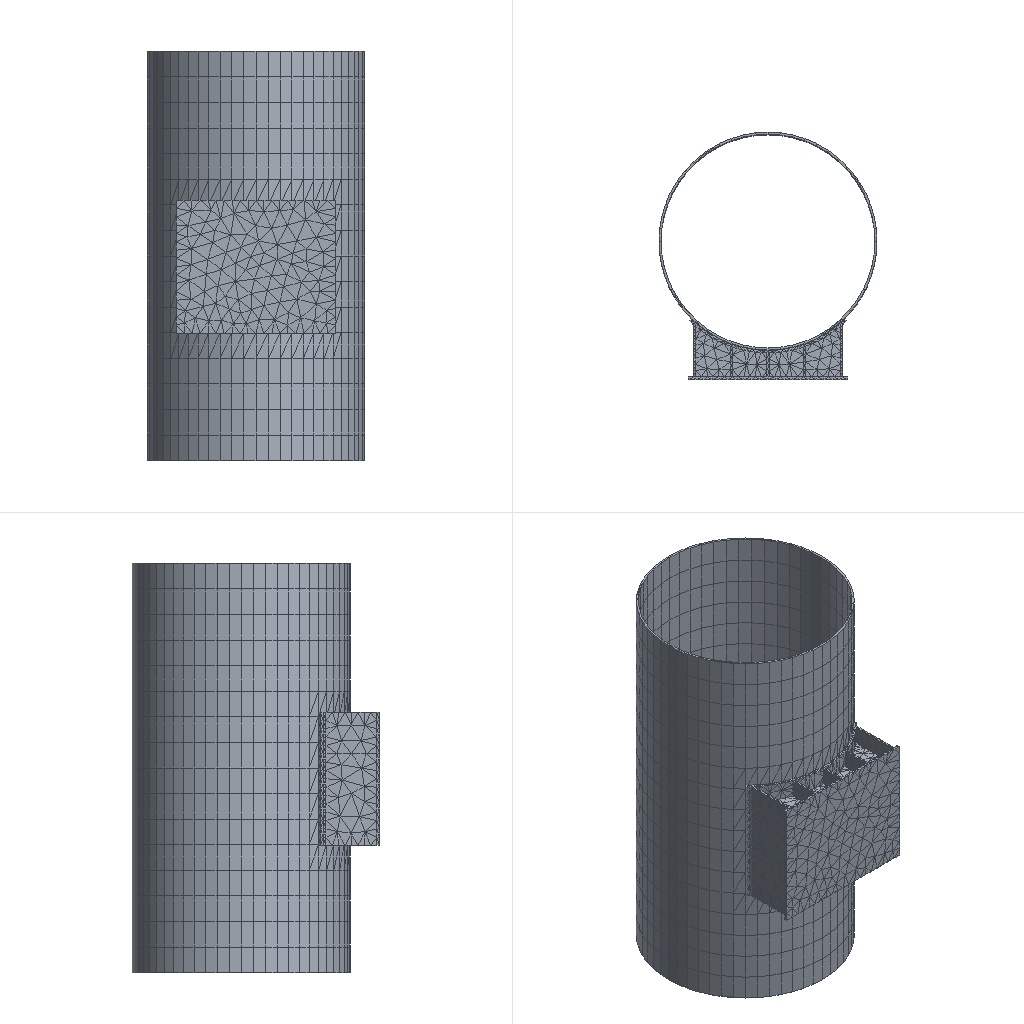Simulation study | ansys workbench
Ansys APDL input file, long lists of numbers shortened:
/batch
/config,noeldb,1     ! force off writing results to database
*get,_wallstrt,active,,time,wall
! ANSYS input file written by Workbench version 2022 R1
! File used for geometry attach:
/title,22222--____ (B5)
! ****** Begin Custom Load Command Snippet ******
/COM, ACT Extensions:
/COM,     LSDYNA, 2021.1
/COM,
! ****** End   Custom Load Command Snippet ******
*DIM,_wb_ProjectScratch_dir,string,248
_wb_ProjectScratch_dir(1) = ''
*DIM,_wb_SolverFiles_dir,string,248
_wb_SolverFiles_dir(1) = ''
*DIM,_wb_userfiles_dir,string,248
_wb_userfiles_dir(1) = ''
/com,--- Data in consistent NMM units. See Solving Units in the help system for more information.
/units,MPA
/nopr
/wb,file,start              !  signify a WB generated input file
/prep7
! Turn off shape checking because checks already performed inside WB mesher.
! See help system for more information.
SHPP,OFF,,NOWARN
/nolist
etcon,set             ! allow ANSYS to choose best KEYOP's for 180x elements, resets any applicable keyopt to MAPDL defaults
/com,*********** Nodes for the whole assembly ***********
nblock,3,,19094
(1i9,3e20.9e3)
        1     2.166365138E+03     3.735729403E+02    -2.923287368E+02
! (17358 more lines like these left out)
-1
/com,*********** Nodes for all Remote Points ***********
nblock,3
(1i9,3e20.9e3)
    17360     1.708271762E+03     2.676707081E+02     9.697962646E+02
    17361     1.708271762E+03     2.676707081E+02     9.697962646E+02
    17362     1.708271762E+03     2.676707081E+02     9.697962646E+02
    17363     1.708271762E+03     2.676707081E+02     9.697962646E+02
    17364     1.708271762E+03     2.676707081E+02     9.697962646E+02
    17365     1.708271762E+03     2.676707081E+02     9.697962646E+02
-1
/wb,elem,start            !  set before creation of elements
/com,*********** Elements for Body 1 "__1^1200-1000|NONE" ***********
et,1,187
eblock,19,solid,,5293
(19i9)
        1        1        1        1        0        0        0        0       10        0     1137     7736     8183     8192     8691    13696    15730    13697    13699
! (10585 more lines like these left out)
-1
/com,*********** Elements for Body 2 "__2^1200-1000|__-__1" ***********
et,2,186
keyo,2,2,1          ! set full integration on SOLID186
eblock,19,solid,,1136
(19i9)
        2        2        2        2        0        0        0        0       20        0        1       16      172     1056     1057      143      548     1475     1474
! (2271 more lines like these left out)
-1
/wb,elem,end               !  done creating elements
/com,*********** Send User Defined Coordinate System(s) ***********
csys,0
toffst,273.15,  ! Temperature offset from absolute zero
/com,*********** Set Reference Temperature ***********
tref,22.
/wb,mat,start              !  starting to send materials
/com,*********** Send Materials ***********
Temperature = 'TEMP' ! Temperature
MP,DENS,1,7.85e-09,	! tonne mm^-3
MP,ALPX,1,1.2e-05,	! C^-1
MP,C,1,434000000,	! mm^2 s^-2 C^-1
MP,KXX,1,60.5,	! tonne mm s^-3 C^-1
MP,RSVX,1,0.00017,	! ohm mm
MP,EX,1,200000,	! tonne s^-2 mm^-1
MP,NUXY,1,0.3,
MP,MURX,1,10000,
Temperature = 'TEMP' ! Temperature
MP,DENS,2,7.85e-09,	! tonne mm^-3
MP,ALPX,2,1.2e-05,	! C^-1
MP,C,2,434000000,	! mm^2 s^-2 C^-1
MP,KXX,2,60.5,	! tonne mm s^-3 C^-1
MP,RSVX,2,0.00017,	! ohm mm
MP,EX,2,200000,	! tonne s^-2 mm^-1
MP,NUXY,2,0.3,
MP,MURX,2,10000,
/wb,mat,end                !  done sending materials
!************************* Model Summary ********************
!__1^1200-1000|NONE,	Q345B,	matid,	1
!__2^1200-1000|__-__1,	Q345B,	matid,	2
!************************* End Model Summary ********************
! get the diagonal of the bounding box. Needed later for other things
*get,_xmin,node,,mnloc,x
*get,_ymin,node,,mnloc,y
*get,_zmin,node,,mnloc,z
*get,_xmax,node,,mxloc,x
*get,_ymax,node,,mxloc,y
*get,_zmax,node,,mxloc,z
_ASMDIAG=(_xmax-_xmin)*(_xmax-_xmin)+(_ymax-_ymin)*(_ymax-_ymin)+(_zmax-_zmin)*(_zmax-_zmin)
_ASMDIAG=SQRT(_ASMDIAG)
/wb,contact,start          !  starting to send contact
/com,*********** Create Contact "接触区域" ***********
/com,            Real Constant Set For Above Contact Is 4 & 3
*set,tid,4
*set,cid,3
r,tid
r,cid
et,tid,170
et,cid,174
eblock,10,,,290
(15i9)
    11634        4        4        4        0     7404     7618     8262     8262    11336    13066     8262    11339
! (289 more lines like these left out)
-1
eblock,10,,,290
(15i9)
    11924        3        3        3        0     7404     7618     8262     8262    11336    13066     8262    11339
! (289 more lines like these left out)
-1
eblock,10,,,112
(15i9)
    12214        3        4        3        0     1163     1164     1137     1136     5519     5469     5466     5467
! (111 more lines like these left out)
-1
eblock,10,,,112
(15i9)
    12326        4        3        4        0     1163     1164     1137     1136     5519     5469     5466     5467
! (111 more lines like these left out)
-1
keyo,cid,8,2               ! auto create asymmetric contact (from Program Controlled setting)
keyo,cid,10,0              ! adjust contact stiffness each NR iteration (from Program Controlled setting)
keyo,cid,12,5              ! bonded always
keyo,cid,18,1              ! small sliding turned on by application
keyo,cid,2,0               ! augmented Lagrange (from Program Controlled setting)
keyo,cid,4,0               ! on Gauss point (from Program Controlled setting)
keyo,cid,9,1               ! ignore initial gaps/penetration
keyo,cid,7,0               ! No Prediction
rmod,tid,3,10.      ! FKN
rmod,tid,5,0.       ! ICONT
rmod,tid,6,0.       ! PINB
rmod,tid,10,0.      ! CNOF
rmod,tid,12,0.      ! FKT
rmod,tid,36,29      ! WB DSID
rmod,cid,3,10.      ! FKN
rmod,cid,5,0.       ! ICONT
rmod,cid,6,0.       ! PINB
rmod,cid,10,0.      ! CNOF
rmod,cid,12,0.      ! FKT
rmod,cid,36,29      ! WB DSID
nsel,all
esel,all
/wb,contact,end            !  done creating contacts
/golist
/wb,load,start             !  starting to send loads
/com,*********** Fixed Supports ***********
CMBLOCK,_FIXEDSU,NODE,     1994
(8i10)
       992      1019      1020      1021      1022      1023      1024      1025
! (249 more lines like these left out)
cmsel,s,_FIXEDSU
d,all,all
nsel,all
/com,*********** Create Remote Point "内部远程点" ***********
! -------- Remote Point Used by "力矩" --------
*set,tid,6
*set,cid,5
et,cid,174
et,tid,170
keyo,tid,2,1               ! Don't fix the pilot node
keyo,tid,4,111111
keyo,cid,12,5              ! Bonded Contact
keyo,cid,4,1               ! Deformable RBE3 style load
keyo,cid,2,2               ! MPC style contact
eblock,10,,,462
(15i9)
    12438        5        5        5        0     8689     8698     8692     8692    17312    17324     8692    17310
! (461 more lines like these left out)
-1
*set,_npilot,17360
_npilot50=_npilot
type,tid
mat ,cid
real,cid
tshape,pilo
en,12900,_npilot
tshape
/com,*********** Create Remote Point "内部远程点" ***********
! -------- Remote Point Used by "力矩 2" --------
*set,tid,8
*set,cid,7
et,cid,174
et,tid,170
keyo,tid,2,1               ! Don't fix the pilot node
keyo,tid,4,111111
keyo,cid,12,5              ! Bonded Contact
keyo,cid,4,1               ! Deformable RBE3 style load
keyo,cid,2,2               ! MPC style contact
eblock,10,,,462
(15i9)
    12901        7        7        7        0     8689     8698     8692     8692    17312    17324     8692    17310
! (461 more lines like these left out)
-1
*set,_npilot,17361
_npilot53=_npilot
type,tid
mat ,cid
real,cid
tshape,pilo
en,13363,_npilot
tshape
/com,*********** Create Remote Point "内部远程点" ***********
! -------- Remote Point Used by "力矩 3" --------
*set,tid,10
*set,cid,9
et,cid,174
et,tid,170
keyo,tid,2,1               ! Don't fix the pilot node
keyo,tid,4,111111
keyo,cid,12,5              ! Bonded Contact
keyo,cid,4,1               ! Deformable RBE3 style load
keyo,cid,2,2               ! MPC style contact
eblock,10,,,462
(15i9)
    13364        9        9        9        0     8689     8698     8692     8692    17312    17324     8692    17310
! (461 more lines like these left out)
-1
*set,_npilot,17362
_npilot56=_npilot
type,tid
mat ,cid
real,cid
tshape,pilo
en,13826,_npilot
tshape
/com,*********** Create Remote Point "内部远程点" ***********
! -------- Remote Point Used by "力矩 4" --------
*set,tid,12
*set,cid,11
et,cid,174
et,tid,170
keyo,tid,2,1               ! Don't fix the pilot node
keyo,tid,4,111111
keyo,cid,12,5              ! Bonded Contact
keyo,cid,4,1               ! Deformable RBE3 style load
keyo,cid,2,2               ! MPC style contact
eblock,10,,,462
(15i9)
    13827       11       11       11        0     8689     8698     8692     8692    17312    17324     8692    17310
! (461 more lines like these left out)
-1
*set,_npilot,17363
_npilot59=_npilot
type,tid
mat ,cid
real,cid
tshape,pilo
en,14289,_npilot
tshape
/com,*********** Create Remote Point "内部远程点" ***********
! -------- Remote Point Used by "力矩 5" --------
*set,tid,14
*set,cid,13
et,cid,174
et,tid,170
keyo,tid,2,1               ! Don't fix the pilot node
keyo,tid,4,111111
keyo,cid,12,5              ! Bonded Contact
keyo,cid,4,1               ! Deformable RBE3 style load
keyo,cid,2,2               ! MPC style contact
eblock,10,,,462
(15i9)
    14290       13       13       13        0     8689     8698     8692     8692    17312    17324     8692    17310
! (461 more lines like these left out)
-1
*set,_npilot,17364
_npilot62=_npilot
type,tid
mat ,cid
real,cid
tshape,pilo
en,14752,_npilot
tshape
/com,*********** Create Remote Point "内部远程点" ***********
! -------- Remote Point Used by "力矩 6" --------
*set,tid,16
*set,cid,15
et,cid,174
et,tid,170
keyo,tid,2,1               ! Don't fix the pilot node
keyo,tid,4,111111
keyo,cid,12,5              ! Bonded Contact
keyo,cid,4,1               ! Deformable RBE3 style load
keyo,cid,2,2               ! MPC style contact
eblock,10,,,462
(15i9)
    14753       15       15       15        0     8689     8698     8692     8692    17312    17324     8692    17310
! (461 more lines like these left out)
-1
*set,_npilot,17365
_npilot65=_npilot
type,tid
mat ,cid
real,cid
tshape,pilo
en,15215,_npilot
tshape
/com,*********** Define Force Using Surface Effect Elements ***********
local,12,0,0.,0.,0.,0.,0.,0.
csys,0
et,17,154
eblock,10,,,290
(15i9)
    15216       17       17       17       12     7404     7618     8262     8262    11336    13066     8262    11339
! (289 more lines like these left out)
-1
esel,s,type,,17
keyop,17,2,1                ! Apply load in local coordinate system
keyop,17,7,1                ! Use original area so load is constant in large deformation
esel,all
/com,*********** Define Force Using Surface Effect Elements ***********
local,13,0,0.,0.,0.,0.,0.,0.
csys,0
et,18,154
eblock,10,,,86
(15i9)
    15506       18       18       18       13     8675     8680     8686     8686    17293    17304     8686    17295
! (85 more lines like these left out)
-1
esel,s,type,,18
keyop,18,2,1                ! Apply load in local coordinate system
keyop,18,7,1                ! Use original area so load is constant in large deformation
esel,all
/com,*********** Define Force Using Surface Effect Elements ***********
local,14,0,0.,0.,0.,0.,0.,0.
csys,0
et,19,154
eblock,10,,,86
(15i9)
    15592       19       19       19       14     8689     8698     8692     8692    17312    17324     8692    17310
! (85 more lines like these left out)
-1
esel,s,type,,19
keyop,19,2,1                ! Apply load in local coordinate system
keyop,19,7,1                ! Use original area so load is constant in large deformation
esel,all
/com,*********** Define Force Using Surface Effect Elements ***********
local,15,0,0.,0.,0.,0.,0.,0.
csys,0
et,20,154
eblock,10,,,112
(15i9)
    15678       20       20       20       15     7077     7659     7873     7873     8888    13243     7873     8889
! (111 more lines like these left out)
-1
esel,s,type,,20
keyop,20,2,1                ! Apply load in local coordinate system
keyop,20,7,1                ! Use original area so load is constant in large deformation
esel,all
/com,*********** Define Force Using Surface Effect Elements ***********
local,16,0,0.,0.,0.,0.,0.,0.
csys,0
et,21,154
eblock,10,,,112
(15i9)
    15790       21       21       21       16     7201     8418     7776     7776     9899    13913     7776     9893
! (111 more lines like these left out)
-1
esel,s,type,,21
keyop,21,2,1                ! Apply load in local coordinate system
keyop,21,7,1                ! Use original area so load is constant in large deformation
esel,all
/com,*********** Construct Moment Using Remote Attachment ***********
/com,*********** Construct Moment Using Remote Attachment ***********
/com,*********** Construct Moment Using Remote Attachment ***********
/com,*********** Construct Moment Using Remote Attachment ***********
/com,*********** Construct Moment Using Remote Attachment ***********
/com,*********** Construct Moment Using Remote Attachment ***********
/gst,on,on
fini
*get,_numnode,node,0,count
*get,_numelem,elem,0,count
*get, _MAXELEMNUM, elem, 0, NUM, MAX
*get, _MAXNODENUM, node, 0, NUM, MAX
*get, _MAXELEMTYPE, etyp, 0, NUM, MAX
*get, _MAXREALCONST, real, 0, NUM, MAX
/go
/wb,load,end               !  done creating loads
/com,--- Number of total nodes = %_numnode%
/com,--- Number of contact elements = 4262
/com,--- Number of spring elements = 0
/com,--- Number of bearing elements = 0
/com,--- Number of solid elements = 6429
/com,--- Number of condensed parts = 0
/com,--- Number of total elements = %_numelem%
*get,_wallbsol,active,,time,wall
/com,****************************************************************************
/com,*************************    SOLUTION       ********************************
/com,****************************************************************************
/solu
antype,0                   ! static analysis
_thickRatio=0.5     ! Ratio of thick parts in the model
eqsl,sparse,,,,,1
cntr,print,1               ! print out contact info and also make no initial contact an error
dmpoption,emat,no             ! Don't combine emat file for DANSYS
dmpoption,esav,no             ! Don't combine esav file for DANSYS
nldiag,cont,iter           ! print out contact info each equilibrium iteration
rescontrol,,none                 ! Do not keep any restart files
/com,****************************************************
/com,******************* SOLVE FOR LS 1 OF 1 ****************
esel,s,type,,17
nsle
sfe,all,1,pres,1,0.
sfe,all,2,pres,1,-0.786
sfe,all,3,pres,1,0.
esel,s,type,,18
nsle
sfe,all,1,pres,1,2.615
sfe,all,2,pres,1,0.
sfe,all,3,pres,1,0.
esel,s,type,,19
nsle
sfe,all,1,pres,1,-2.615
sfe,all,2,pres,1,0.
sfe,all,3,pres,1,0.
esel,s,type,,20
nsle
sfe,all,1,pres,1,0.
sfe,all,2,pres,1,0.
sfe,all,3,pres,1,-0.985
esel,s,type,,21
nsle
sfe,all,1,pres,1,0.
sfe,all,2,pres,1,0.
sfe,all,3,pres,1,0.985
nsel,all
esel,all
nsel,s,node,,17360
f,all,mx,120000.
f,all,my,0.
f,all,mz,0.
nsel,s,node,,17361
f,all,mx,-120000.
f,all,my,0.
f,all,mz,0.
nsel,s,node,,17362
f,all,mx,0.
f,all,my,1200000.
f,all,mz,0.
nsel,s,node,,17363
f,all,mx,0.
f,all,my,-1200000.
f,all,mz,0.
nsel,s,node,,17364
f,all,mx,0.
f,all,my,0.
f,all,mz,1400000.
nsel,s,node,,17365
f,all,mx,0.
f,all,my,0.
f,all,mz,-1400000.
nsel,all
/nopr
/gopr
nsub,1,1,1
time,1.
outres,erase
outres,all,none
outres,nsol,all,
outres,rsol,all
outres,eangl,all
outres,etmp,all
outres,veng,all
outres,strs,all,
outres,epel,all,
outres,eppl,all,
outres,cont,all,
! *********** WB SOLVE COMMAND ***********
! check interactive state
*get,ANSINTER_,active,,int
*if,ANSINTER_,ne,0,then
/eof
*endif
solve
/com *************** Write FE CONNECTORS *********
CEWRITE,file,ce,,INTE
/com,****************************************************
/com,*************** FINISHED SOLVE FOR LS 1 *************
*get,_wallasol,active,,time,wall
/nopr
*get,_numnode,node,0,count
*get,_numelem,elem,0,count
*get, _MAXELEMNUM, elem, 0, NUM, MAX
*get, _MAXNODENUM, node, 0, NUM, MAX,,,INTERNAL
*get, _MAXELEMTYPE, etyp, 0, NUM, MAX
*get, _MAXREALCONST, real, 0, NUM, MAX
/gopr
/post1
xmlo,ENCODING,ISO-8859-1
xmlo,parm
/xml,parm,xml
fini
/gopr
*get,_walldone,active,,time,wall
_preptime=(_wallbsol-_wallstrt)*3600
_solvtime=(_wallasol-_wallbsol)*3600
_posttime=(_walldone-_wallasol)*3600
_totaltim=(_walldone-_wallstrt)*3600
*get,_dlbratio,active,0,solu,dlbr
*get,_combtime,active,0,solu,comb
*get,_ssmode,active,0,solu,ssmm
*get,_ndofs,active,0,solu,ndof
*get,_sol_end_time,active,0,set,time
*if,_sol_end_time,eq,1.,then
/fclean				!clean distributed files
*endif
/com,--- Total number of nodes = %_numnode%
/com,--- Total number of elements = %_numelem%
/com,--- Element load balance ratio = %_dlbratio%
/com,--- Time to combine distributed files = %_combtime%
/com,--- Sparse memory mode = %_ssmode%
/com,--- Number of DOF = %_ndofs%
/wb,file,end               ! done with WB generated input